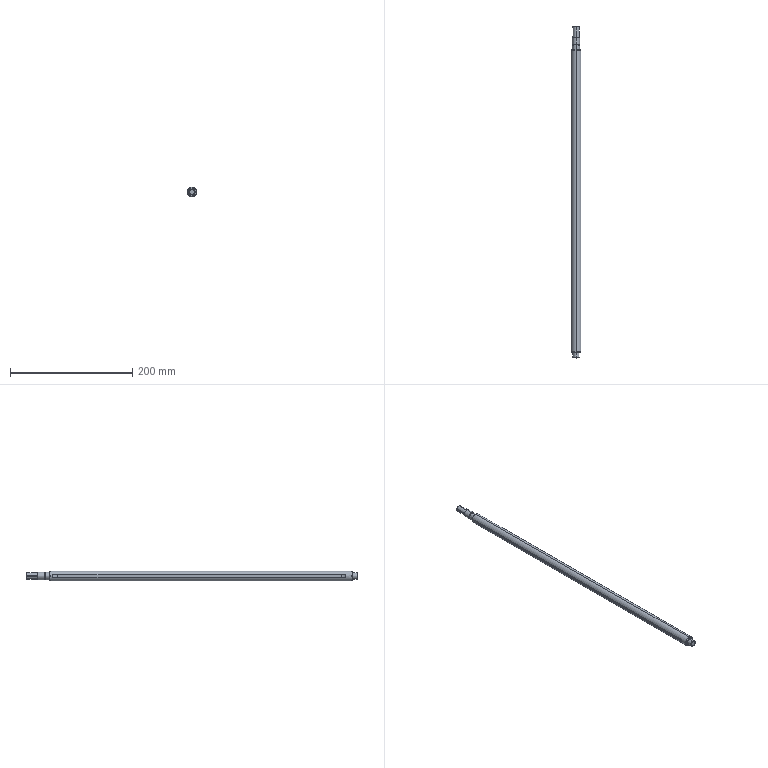Part | STEP file | Drive shaft 2 | 1 solid | 37 faces | box 16 x 544 x 16 mm | volume 100395 mm3 | cylinder 14 | plane 13 | cone 8 | spline 2 | commonest cylinder face diameters 10 x4 12 x4 3 x2 11.2 x2 16 x2